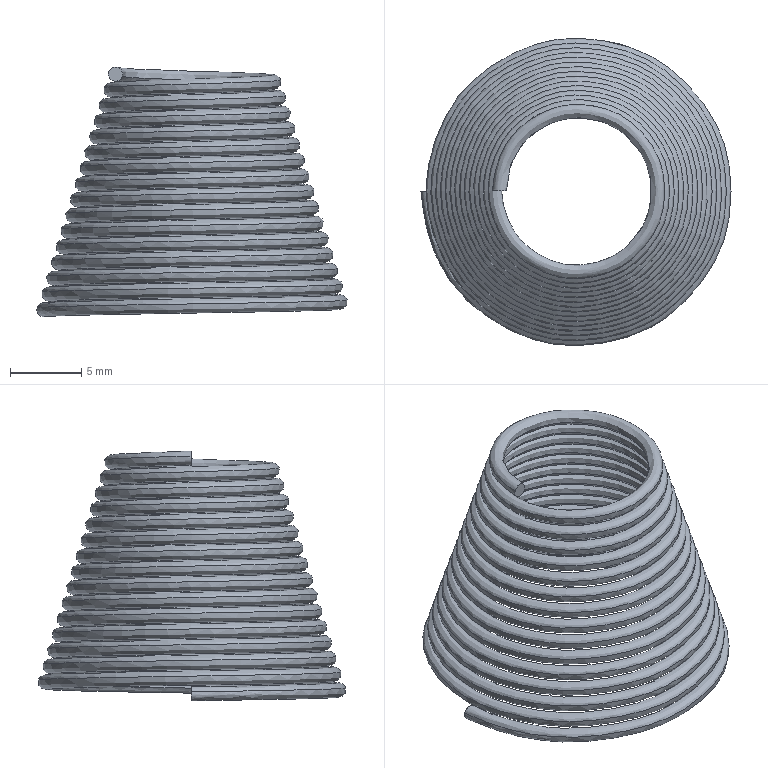Part | SolidWorks | features BaseBody 1 | 1 solid | 4 faces | box 21.728 x 21.559 x 17.499 mm | volume 589.39 mm3 | spline 2 | plane 2